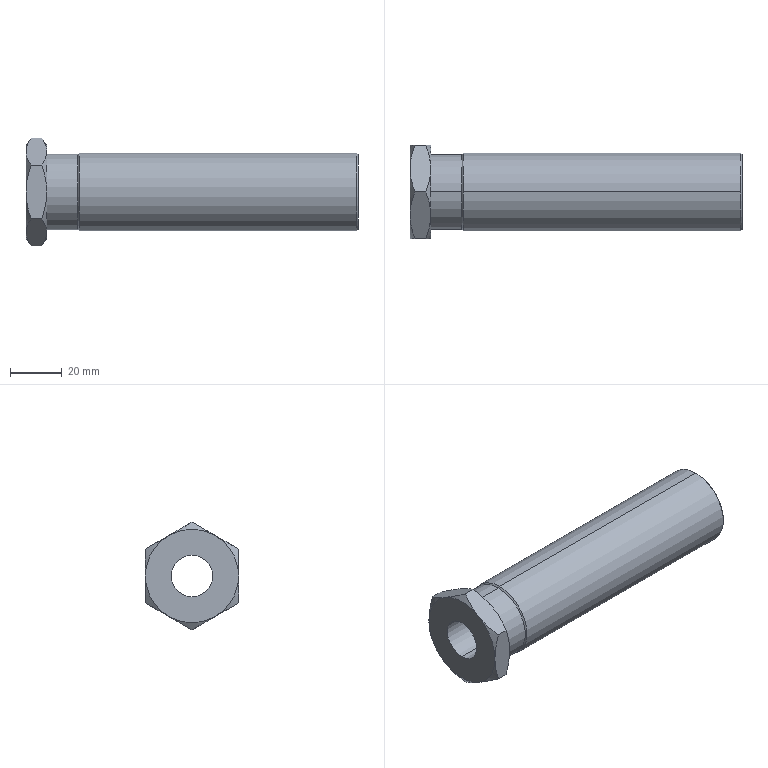Part | SolidWorks | features ICE 2, Extrusion 1, RevCut 1, Revolution 1 | 1 solid | 32 faces | box 128 x 36 x 41.569 mm | volume 67364 mm3 | cone 17 | plane 9 | cylinder 6 | commonest cylinder face diameters 16 x2 29 x2 30 x2
STEP:
#1=CARTESIAN_POINT('',(120.,0.,-8.));
#2=VERTEX_POINT('',#1);
#3=CARTESIAN_POINT('',(120.,0.,8.));
#4=VERTEX_POINT('',#3);
#5=CARTESIAN_POINT('',(120.,0.,0.));
#6=DIRECTION('',(-1.,0.,0.));
#7=DIRECTION('',(0.,0.,1.));
#8=AXIS2_PLACEMENT_3D('',#5,#6,#7);
#9=CIRCLE('',#8,8.);
#10=EDGE_CURVE('',#2,#4,#9,.T.);
#11=ORIENTED_EDGE('',*,*,#10,.F.);
#12=CARTESIAN_POINT('',(-8.,0.,-8.));
#13=VERTEX_POINT('',#12);
#14=CARTESIAN_POINT('',(0.,0.,-8.));
#15=DIRECTION('',(-1.,0.,0.));
#16=VECTOR('',#15,1000.);
#17=LINE('',#14,#16);
#18=EDGE_CURVE('',#2,#13,#17,.T.);
#19=ORIENTED_EDGE('',*,*,#18,.T.);
#20=CARTESIAN_POINT('',(-8.,0.,8.));
#21=VERTEX_POINT('',#20);
#22=CARTESIAN_POINT('',(-8.,0.,0.));
#23=DIRECTION('',(-1.,0.,0.));
#24=DIRECTION('',(0.,0.,1.));
#25=AXIS2_PLACEMENT_3D('',#22,#23,#24);
#26=CIRCLE('',#25,8.);
#27=EDGE_CURVE('',#13,#21,#26,.T.);
#28=ORIENTED_EDGE('',*,*,#27,.T.);
#29=CARTESIAN_POINT('',(0.,0.,8.));
#30=DIRECTION('',(-1.,0.,0.));
#31=VECTOR('',#30,1000.);
#32=LINE('',#29,#31);
#33=EDGE_CURVE('',#4,#21,#32,.T.);
#34=ORIENTED_EDGE('',*,*,#33,.F.);
#35=EDGE_LOOP('',(#11,#19,#28,#34));
#36=FACE_OUTER_BOUND('',#35,.T.);
#37=CARTESIAN_POINT('',(0.,0.,0.));
#38=DIRECTION('',(-1.,0.,0.));
#39=DIRECTION('',(0.,0.,1.));
#40=AXIS2_PLACEMENT_3D('',#37,#38,#39);
#41=CYLINDRICAL_SURFACE('',#40,8.);
#42=ADVANCED_FACE('',(#36),#41,.F.);
#43=CARTESIAN_POINT('',(0.,9.,-15.588));
#44=VERTEX_POINT('',#43);
#45=CARTESIAN_POINT('',(0.,0.,-18.));
#46=VERTEX_POINT('',#45);
#47=CARTESIAN_POINT('',(0.,0.,0.));
#48=DIRECTION('',(-1.,0.,0.));
#49=DIRECTION('',(0.,0.,1.));
#50=AXIS2_PLACEMENT_3D('',#47,#48,#49);
#51=CIRCLE('',#50,18.);
#52=EDGE_CURVE('',#44,#46,#51,.T.);
#53=ORIENTED_EDGE('',*,*,#52,.T.);
#54=CARTESIAN_POINT('',(-1.95,0.,-20.785));
#55=VERTEX_POINT('',#54);
#56=CARTESIAN_POINT('',(0.,0.,-18.));
#57=DIRECTION('',(-0.5736,0.,-0.8192));
#58=VECTOR('',#57,1000.);
#59=LINE('',#56,#58);
#60=EDGE_CURVE('',#46,#55,#59,.T.);
#61=ORIENTED_EDGE('',*,*,#60,.T.);
#62=CARTESIAN_POINT('',(-1.95,0.,-20.785));
#63=CARTESIAN_POINT('',(-1.359,1.461,-19.941));
#64=CARTESIAN_POINT('',(-0.8697,2.937,-19.089));
#65=CARTESIAN_POINT('',(-0.189,5.933,-17.359));
#66=CARTESIAN_POINT('',(0.,7.453,-16.482));
#67=CARTESIAN_POINT('',(0.,9.,-15.588));
#68=B_SPLINE_CURVE_WITH_KNOTS('',3,(#62,#63,#64,#65,#66,#67),.UNSPECIFIED.,.F.,.F.,(4,2,4),(0.000000241,0.005286,0.01057),.UNSPECIFIED.);
#69=EDGE_CURVE('',#55,#44,#68,.T.);
#70=ORIENTED_EDGE('',*,*,#69,.T.);
#71=EDGE_LOOP('',(#53,#61,#70));
#72=FACE_OUTER_BOUND('',#71,.T.);
#73=CARTESIAN_POINT('',(0.,0.,0.));
#74=DIRECTION('',(-1.,0.,0.));
#75=DIRECTION('',(0.,0.,-1.));
#76=AXIS2_PLACEMENT_3D('',#73,#74,#75);
#77=CONICAL_SURFACE('',#76,18.,0.9599);
#78=ADVANCED_FACE('',(#72),#77,.T.);
#79=CARTESIAN_POINT('',(12.,0.,14.5));
#80=VERTEX_POINT('',#79);
#81=CARTESIAN_POINT('',(12.,0.,-14.5));
#82=VERTEX_POINT('',#81);
#83=CARTESIAN_POINT('',(12.,0.,0.));
#84=DIRECTION('',(-1.,0.,0.));
#85=DIRECTION('',(0.,0.,1.));
#86=AXIS2_PLACEMENT_3D('',#83,#84,#85);
#87=CIRCLE('',#86,14.5);
#88=EDGE_CURVE('',#80,#82,#87,.T.);
#89=ORIENTED_EDGE('',*,*,#88,.T.);
#90=CARTESIAN_POINT('',(0.,0.,-14.5));
#91=VERTEX_POINT('',#90);
#92=CARTESIAN_POINT('',(0.,0.,-14.5));
#93=DIRECTION('',(-1.,0.,0.));
#94=VECTOR('',#93,1000.);
#95=LINE('',#92,#94);
#96=EDGE_CURVE('',#82,#91,#95,.T.);
#97=ORIENTED_EDGE('',*,*,#96,.T.);
#98=CARTESIAN_POINT('',(0.,0.,14.5));
#99=VERTEX_POINT('',#98);
#100=CARTESIAN_POINT('',(0.,0.,0.));
#101=DIRECTION('',(-1.,0.,0.));
#102=DIRECTION('',(0.,0.,1.));
#103=AXIS2_PLACEMENT_3D('',#100,#101,#102);
#104=CIRCLE('',#103,14.5);
#105=EDGE_CURVE('',#99,#91,#104,.T.);
#106=ORIENTED_EDGE('',*,*,#105,.F.);
#107=CARTESIAN_POINT('',(0.,0.,14.5));
#108=DIRECTION('',(-1.,0.,0.));
#109=VECTOR('',#108,1000.);
#110=LINE('',#107,#109);
#111=EDGE_CURVE('',#80,#99,#110,.T.);
#112=ORIENTED_EDGE('',*,*,#111,.F.);
#113=EDGE_LOOP('',(#89,#97,#106,#112));
#114=FACE_OUTER_BOUND('',#113,.T.);
#115=CARTESIAN_POINT('',(0.,0.,0.));
#116=DIRECTION('',(-1.,0.,0.));
#117=DIRECTION('',(0.,0.,1.));
#118=AXIS2_PLACEMENT_3D('',#115,#116,#117);
#119=CYLINDRICAL_SURFACE('',#118,14.5);
#120=ADVANCED_FACE('',(#114),#119,.T.);
#121=ORIENTED_EDGE('',*,*,#88,.F.);
#122=CARTESIAN_POINT('',(12.5,0.,15.));
#123=VERTEX_POINT('',#122);
#124=CARTESIAN_POINT('',(12.5,0.,15.));
#125=DIRECTION('',(0.7071,0.,0.7071));
#126=VECTOR('',#125,1000.);
#127=LINE('',#124,#126);
#128=EDGE_CURVE('',#80,#123,#127,.T.);
#129=ORIENTED_EDGE('',*,*,#128,.T.);
#130=CARTESIAN_POINT('',(12.5,0.,-15.));
#131=VERTEX_POINT('',#130);
#132=CARTESIAN_POINT('',(12.5,0.,0.));
#133=DIRECTION('',(-1.,0.,0.));
#134=DIRECTION('',(0.,0.,1.));
#135=AXIS2_PLACEMENT_3D('',#132,#133,#134);
#136=CIRCLE('',#135,15.);
#137=EDGE_CURVE('',#123,#131,#136,.T.);
#138=ORIENTED_EDGE('',*,*,#137,.T.);
#139=CARTESIAN_POINT('',(12.5,0.,-15.));
#140=DIRECTION('',(0.7071,0.,-0.7071));
#141=VECTOR('',#140,1000.);
#142=LINE('',#139,#141);
#143=EDGE_CURVE('',#82,#131,#142,.T.);
#144=ORIENTED_EDGE('',*,*,#143,.F.);
#145=EDGE_LOOP('',(#121,#129,#138,#144));
#146=FACE_OUTER_BOUND('',#145,.T.);
#147=CARTESIAN_POINT('',(12.5,0.,0.));
#148=DIRECTION('',(1.,0.,0.));
#149=DIRECTION('',(0.,0.,-1.));
#150=AXIS2_PLACEMENT_3D('',#147,#148,#149);
#151=CONICAL_SURFACE('',#150,15.,0.7854);
#152=ADVANCED_FACE('',(#146),#151,.T.);
#153=CARTESIAN_POINT('',(119.5,0.,15.));
#154=VERTEX_POINT('',#153);
#155=CARTESIAN_POINT('',(119.5,0.,-15.));
#156=VERTEX_POINT('',#155);
#157=CARTESIAN_POINT('',(119.5,0.,0.));
#158=DIRECTION('',(-1.,0.,0.));
#159=DIRECTION('',(0.,0.,1.));
#160=AXIS2_PLACEMENT_3D('',#157,#158,#159);
#161=CIRCLE('',#160,15.);
#162=EDGE_CURVE('',#154,#156,#161,.T.);
#163=ORIENTED_EDGE('',*,*,#162,.T.);
#164=CARTESIAN_POINT('',(0.,0.,-15.));
#165=DIRECTION('',(-1.,0.,0.));
#166=VECTOR('',#165,1000.);
#167=LINE('',#164,#166);
#168=EDGE_CURVE('',#156,#131,#167,.T.);
#169=ORIENTED_EDGE('',*,*,#168,.T.);
#170=ORIENTED_EDGE('',*,*,#137,.F.);
#171=CARTESIAN_POINT('',(0.,0.,15.));
#172=DIRECTION('',(-1.,0.,0.));
#173=VECTOR('',#172,1000.);
#174=LINE('',#171,#173);
#175=EDGE_CURVE('',#154,#123,#174,.T.);
#176=ORIENTED_EDGE('',*,*,#175,.F.);
#177=EDGE_LOOP('',(#163,#169,#170,#176));
#178=FACE_OUTER_BOUND('',#177,.T.);
#179=CARTESIAN_POINT('',(0.,0.,0.));
#180=DIRECTION('',(-1.,0.,0.));
#181=DIRECTION('',(0.,0.,1.));
#182=AXIS2_PLACEMENT_3D('',#179,#180,#181);
#183=CYLINDRICAL_SURFACE('',#182,15.);
#184=ADVANCED_FACE('',(#178),#183,.T.);
#185=CARTESIAN_POINT('',(120.,0.,14.5));
#186=VERTEX_POINT('',#185);
#187=CARTESIAN_POINT('',(120.,0.,-14.5));
#188=VERTEX_POINT('',#187);
#189=CARTESIAN_POINT('',(120.,0.,0.));
#190=DIRECTION('',(-1.,0.,0.));
#191=DIRECTION('',(0.,0.,1.));
#192=AXIS2_PLACEMENT_3D('',#189,#190,#191);
#193=CIRCLE('',#192,14.5);
#194=EDGE_CURVE('',#186,#188,#193,.T.);
#195=ORIENTED_EDGE('',*,*,#194,.T.);
#196=CARTESIAN_POINT('',(120.,0.,-14.5));
#197=DIRECTION('',(-0.7071,0.,-0.7071));
#198=VECTOR('',#197,1000.);
#199=LINE('',#196,#198);
#200=EDGE_CURVE('',#188,#156,#199,.T.);
#201=ORIENTED_EDGE('',*,*,#200,.T.);
#202=ORIENTED_EDGE('',*,*,#162,.F.);
#203=CARTESIAN_POINT('',(120.,0.,14.5));
#204=DIRECTION('',(-0.7071,0.,0.7071));
#205=VECTOR('',#204,1000.);
#206=LINE('',#203,#205);
#207=EDGE_CURVE('',#186,#154,#206,.T.);
#208=ORIENTED_EDGE('',*,*,#207,.F.);
#209=EDGE_LOOP('',(#195,#201,#202,#208));
#210=FACE_OUTER_BOUND('',#209,.T.);
#211=CARTESIAN_POINT('',(120.,0.,0.));
#212=DIRECTION('',(-1.,0.,0.));
#213=DIRECTION('',(0.,0.,1.));
#214=AXIS2_PLACEMENT_3D('',#211,#212,#213);
#215=CONICAL_SURFACE('',#214,14.5,0.7854);
#216=ADVANCED_FACE('',(#210),#215,.T.);
#217=ORIENTED_EDGE('',*,*,#194,.F.);
#218=CARTESIAN_POINT('',(120.,0.,0.));
#219=DIRECTION('',(-1.,0.,0.));
#220=DIRECTION('',(0.,0.,1.));
#221=AXIS2_PLACEMENT_3D('',#218,#219,#220);
#222=CIRCLE('',#221,14.5);
#223=EDGE_CURVE('',#188,#186,#222,.T.);
#224=ORIENTED_EDGE('',*,*,#223,.F.);
#225=EDGE_LOOP('',(#217,#224));
#226=FACE_OUTER_BOUND('',#225,.T.);
#227=CARTESIAN_POINT('',(120.,0.,0.));
#228=DIRECTION('',(-1.,0.,0.));
#229=DIRECTION('',(0.,0.,1.));
#230=AXIS2_PLACEMENT_3D('',#227,#228,#229);
#231=CIRCLE('',#230,8.);
#232=EDGE_CURVE('',#4,#2,#231,.T.);
#233=ORIENTED_EDGE('',*,*,#232,.T.);
#234=ORIENTED_EDGE('',*,*,#10,.T.);
#235=EDGE_LOOP('',(#233,#234));
#236=FACE_BOUND('',#235,.T.);
#237=CARTESIAN_POINT('',(120.,0.,0.));
#238=DIRECTION('',(-1.,0.,0.));
#239=DIRECTION('',(0.,0.,1.));
#240=AXIS2_PLACEMENT_3D('',#237,#238,#239);
#241=PLANE('',#240);
#242=ADVANCED_FACE('',(#226,#236),#241,.F.);
#243=CARTESIAN_POINT('',(-8.,-9.,15.588));
#244=VERTEX_POINT('',#243);
#245=CARTESIAN_POINT('',(-8.,9.,15.588));
#246=VERTEX_POINT('',#245);
#247=CARTESIAN_POINT('',(-8.,0.,0.));
#248=DIRECTION('',(-1.,0.,0.));
#249=DIRECTION('',(0.,0.,1.));
#250=AXIS2_PLACEMENT_3D('',#247,#248,#249);
#251=CIRCLE('',#250,18.);
#252=EDGE_CURVE('',#244,#246,#251,.T.);
#253=ORIENTED_EDGE('',*,*,#252,.T.);
#254=CARTESIAN_POINT('',(-8.,18.,0.));
#255=VERTEX_POINT('',#254);
#256=CARTESIAN_POINT('',(-8.,0.,0.));
#257=DIRECTION('',(-1.,0.,0.));
#258=DIRECTION('',(0.,0.,1.));
#259=AXIS2_PLACEMENT_3D('',#256,#257,#258);
#260=CIRCLE('',#259,18.);
#261=EDGE_CURVE('',#246,#255,#260,.T.);
#262=ORIENTED_EDGE('',*,*,#261,.T.);
#263=CARTESIAN_POINT('',(-8.,9.,-15.588));
#264=VERTEX_POINT('',#263);
#265=CARTESIAN_POINT('',(-8.,0.,0.));
#266=DIRECTION('',(-1.,0.,0.));
#267=DIRECTION('',(0.,0.,1.));
#268=AXIS2_PLACEMENT_3D('',#265,#266,#267);
#269=CIRCLE('',#268,18.);
#270=EDGE_CURVE('',#255,#264,#269,.T.);
#271=ORIENTED_EDGE('',*,*,#270,.T.);
#272=CARTESIAN_POINT('',(-8.,-9.,-15.588));
#273=VERTEX_POINT('',#272);
#274=CARTESIAN_POINT('',(-8.,0.,0.));
#275=DIRECTION('',(-1.,0.,0.));
#276=DIRECTION('',(0.,0.,1.));
#277=AXIS2_PLACEMENT_3D('',#274,#275,#276);
#278=CIRCLE('',#277,18.);
#279=EDGE_CURVE('',#264,#273,#278,.T.);
#280=ORIENTED_EDGE('',*,*,#279,.T.);
#281=CARTESIAN_POINT('',(-8.,-18.,0.));
#282=VERTEX_POINT('',#281);
#283=CARTESIAN_POINT('',(-8.,0.,0.));
#284=DIRECTION('',(-1.,0.,0.));
#285=DIRECTION('',(0.,0.,1.));
#286=AXIS2_PLACEMENT_3D('',#283,#284,#285);
#287=CIRCLE('',#286,18.);
#288=EDGE_CURVE('',#273,#282,#287,.T.);
#289=ORIENTED_EDGE('',*,*,#288,.T.);
#290=CARTESIAN_POINT('',(-8.,0.,0.));
#291=DIRECTION('',(-1.,0.,0.));
#292=DIRECTION('',(0.,-1.,0.));
#293=AXIS2_PLACEMENT_3D('',#290,#291,#292);
#294=CIRCLE('',#293,18.);
#295=EDGE_CURVE('',#282,#244,#294,.T.);
#296=ORIENTED_EDGE('',*,*,#295,.T.);
#297=EDGE_LOOP('',(#253,#262,#271,#280,#289,#296));
#298=FACE_OUTER_BOUND('',#297,.T.);
#299=CARTESIAN_POINT('',(-8.,0.,0.));
#300=DIRECTION('',(-1.,0.,0.));
#301=DIRECTION('',(0.,0.,1.));
#302=AXIS2_PLACEMENT_3D('',#299,#300,#301);
#303=CIRCLE('',#302,8.);
#304=EDGE_CURVE('',#21,#13,#303,.T.);
#305=ORIENTED_EDGE('',*,*,#304,.F.);
#306=ORIENTED_EDGE('',*,*,#27,.F.);
#307=EDGE_LOOP('',(#305,#306));
#308=FACE_BOUND('',#307,.T.);
#309=CARTESIAN_POINT('',(-8.,0.,-20.785));
#310=DIRECTION('',(-1.,0.,0.));
#311=DIRECTION('',(0.,0.,1.));
#312=AXIS2_PLACEMENT_3D('',#309,#310,#311);
#313=PLANE('',#312);
#314=ADVANCED_FACE('',(#298,#308),#313,.T.);
#315=ORIENTED_EDGE('',*,*,#105,.T.);
#316=CARTESIAN_POINT('',(0.,0.,0.));
#317=DIRECTION('',(-1.,0.,0.));
#318=DIRECTION('',(0.,0.,1.));
#319=AXIS2_PLACEMENT_3D('',#316,#317,#318);
#320=CIRCLE('',#319,14.5);
#321=EDGE_CURVE('',#91,#99,#320,.T.);
#322=ORIENTED_EDGE('',*,*,#321,.T.);
#323=EDGE_LOOP('',(#315,#322));
#324=FACE_BOUND('',#323,.T.);
#325=CARTESIAN_POINT('',(0.,9.,15.588));
#326=VERTEX_POINT('',#325);
#327=CARTESIAN_POINT('',(0.,18.,0.));
#328=VERTEX_POINT('',#327);
#329=CARTESIAN_POINT('',(0.,0.,0.));
#330=DIRECTION('',(-1.,0.,0.));
#331=DIRECTION('',(0.,0.,1.));
#332=AXIS2_PLACEMENT_3D('',#329,#330,#331);
#333=CIRCLE('',#332,18.);
#334=EDGE_CURVE('',#326,#328,#333,.T.);
#335=ORIENTED_EDGE('',*,*,#334,.F.);
#336=CARTESIAN_POINT('',(0.,-9.,15.588));
#337=VERTEX_POINT('',#336);
#338=CARTESIAN_POINT('',(0.,0.,0.));
#339=DIRECTION('',(-1.,0.,0.));
#340=DIRECTION('',(0.,0.,1.));
#341=AXIS2_PLACEMENT_3D('',#338,#339,#340);
#342=CIRCLE('',#341,18.);
#343=EDGE_CURVE('',#337,#326,#342,.T.);
#344=ORIENTED_EDGE('',*,*,#343,.F.);
#345=CARTESIAN_POINT('',(0.,-18.,0.));
#346=VERTEX_POINT('',#345);
#347=CARTESIAN_POINT('',(0.,0.,0.));
#348=DIRECTION('',(-1.,0.,0.));
#349=DIRECTION('',(0.,0.,1.));
#350=AXIS2_PLACEMENT_3D('',#347,#348,#349);
#351=CIRCLE('',#350,18.);
#352=EDGE_CURVE('',#346,#337,#351,.T.);
#353=ORIENTED_EDGE('',*,*,#352,.F.);
#354=CARTESIAN_POINT('',(0.,-9.,-15.588));
#355=VERTEX_POINT('',#354);
#356=CARTESIAN_POINT('',(0.,0.,0.));
#357=DIRECTION('',(-1.,0.,0.));
#358=DIRECTION('',(0.,0.,1.));
#359=AXIS2_PLACEMENT_3D('',#356,#357,#358);
#360=CIRCLE('',#359,18.);
#361=EDGE_CURVE('',#355,#346,#360,.T.);
#362=ORIENTED_EDGE('',*,*,#361,.F.);
#363=CARTESIAN_POINT('',(0.,0.,0.));
#364=DIRECTION('',(-1.,0.,0.));
#365=DIRECTION('',(0.,0.,1.));
#366=AXIS2_PLACEMENT_3D('',#363,#364,#365);
#367=CIRCLE('',#366,18.);
#368=EDGE_CURVE('',#46,#355,#367,.T.);
#369=ORIENTED_EDGE('',*,*,#368,.F.);
#370=ORIENTED_EDGE('',*,*,#52,.F.);
#371=CARTESIAN_POINT('',(0.,0.,0.));
#372=DIRECTION('',(1.,0.,0.));
#373=DIRECTION('',(0.,0.,-1.));
#374=AXIS2_PLACEMENT_3D('',#371,#372,#373);
#375=CIRCLE('',#374,18.);
#376=EDGE_CURVE('',#44,#328,#375,.T.);
#377=ORIENTED_EDGE('',*,*,#376,.T.);
#378=EDGE_LOOP('',(#335,#344,#353,#362,#369,#370,#377));
#379=FACE_OUTER_BOUND('',#378,.T.);
#380=CARTESIAN_POINT('',(0.,0.,-20.785));
#381=DIRECTION('',(-1.,0.,0.));
#382=DIRECTION('',(0.,0.,1.));
#383=AXIS2_PLACEMENT_3D('',#380,#381,#382);
#384=PLANE('',#383);
#385=ADVANCED_FACE('',(#324,#379),#384,.F.);
#386=ORIENTED_EDGE('',*,*,#200,.F.);
#387=ORIENTED_EDGE('',*,*,#223,.T.);
#388=ORIENTED_EDGE('',*,*,#207,.T.);
#389=CARTESIAN_POINT('',(119.5,0.,0.));
#390=DIRECTION('',(-1.,0.,0.));
#391=DIRECTION('',(0.,0.,1.));
#392=AXIS2_PLACEMENT_3D('',#389,#390,#391);
#393=CIRCLE('',#392,15.);
#394=EDGE_CURVE('',#156,#154,#393,.T.);
#395=ORIENTED_EDGE('',*,*,#394,.F.);
#396=EDGE_LOOP('',(#386,#387,#388,#395));
#397=FACE_OUTER_BOUND('',#396,.T.);
#398=CARTESIAN_POINT('',(120.,0.,0.));
#399=DIRECTION('',(-1.,0.,0.));
#400=DIRECTION('',(0.,0.,1.));
#401=AXIS2_PLACEMENT_3D('',#398,#399,#400);
#402=CONICAL_SURFACE('',#401,14.5,0.7854);
#403=ADVANCED_FACE('',(#397),#402,.T.);
#404=ORIENTED_EDGE('',*,*,#168,.F.);
#405=ORIENTED_EDGE('',*,*,#394,.T.);
#406=ORIENTED_EDGE('',*,*,#175,.T.);
#407=CARTESIAN_POINT('',(12.5,0.,0.));
#408=DIRECTION('',(-1.,0.,0.));
#409=DIRECTION('',(0.,0.,1.));
#410=AXIS2_PLACEMENT_3D('',#407,#408,#409);
#411=CIRCLE('',#410,15.);
#412=EDGE_CURVE('',#131,#123,#411,.T.);
#413=ORIENTED_EDGE('',*,*,#412,.F.);
#414=EDGE_LOOP('',(#404,#405,#406,#413));
#415=FACE_OUTER_BOUND('',#414,.T.);
#416=CARTESIAN_POINT('',(0.,0.,0.));
#417=DIRECTION('',(-1.,0.,0.));
#418=DIRECTION('',(0.,0.,1.));
#419=AXIS2_PLACEMENT_3D('',#416,#417,#418);
#420=CYLINDRICAL_SURFACE('',#419,15.);
#421=ADVANCED_FACE('',(#415),#420,.T.);
#422=ORIENTED_EDGE('',*,*,#128,.F.);
#423=CARTESIAN_POINT('',(12.,0.,0.));
#424=DIRECTION('',(-1.,0.,0.));
#425=DIRECTION('',(0.,0.,1.));
#426=AXIS2_PLACEMENT_3D('',#423,#424,#425);
#427=CIRCLE('',#426,14.5);
#428=EDGE_CURVE('',#82,#80,#427,.T.);
#429=ORIENTED_EDGE('',*,*,#428,.F.);
#430=ORIENTED_EDGE('',*,*,#143,.T.);
#431=ORIENTED_EDGE('',*,*,#412,.T.);
#432=EDGE_LOOP('',(#422,#429,#430,#431));
#433=FACE_OUTER_BOUND('',#432,.T.);
#434=CARTESIAN_POINT('',(12.5,0.,0.));
#435=DIRECTION('',(1.,0.,0.));
#436=DIRECTION('',(0.,0.,-1.));
#437=AXIS2_PLACEMENT_3D('',#434,#435,#436);
#438=CONICAL_SURFACE('',#437,15.,0.7854);
#439=ADVANCED_FACE('',(#433),#438,.T.);
#440=ORIENTED_EDGE('',*,*,#96,.F.);
#441=ORIENTED_EDGE('',*,*,#428,.T.);
#442=ORIENTED_EDGE('',*,*,#111,.T.);
#443=ORIENTED_EDGE('',*,*,#321,.F.);
#444=EDGE_LOOP('',(#440,#441,#442,#443));
#445=FACE_OUTER_BOUND('',#444,.T.);
#446=CARTESIAN_POINT('',(0.,0.,0.));
#447=DIRECTION('',(-1.,0.,0.));
#448=DIRECTION('',(0.,0.,1.));
#449=AXIS2_PLACEMENT_3D('',#446,#447,#448);
#450=CYLINDRICAL_SURFACE('',#449,14.5);
#451=ADVANCED_FACE('',(#445),#450,.T.);
#452=CARTESIAN_POINT('',(-1.95,0.,20.785));
#453=VERTEX_POINT('',#452);
#454=CARTESIAN_POINT('',(-1.95,0.,20.785));
#455=CARTESIAN_POINT('',(-1.359,-1.461,19.941));
#456=CARTESIAN_POINT('',(-0.8697,-2.937,19.089));
#457=CARTESIAN_POINT('',(-0.189,-5.933,17.359));
#458=CARTESIAN_POINT('',(0.,-7.453,16.482));
#459=CARTESIAN_POINT('',(0.,-9.,15.588));
#460=B_SPLINE_CURVE_WITH_KNOTS('',3,(#454,#455,#456,#457,#458,#459),.UNSPECIFIED.,.F.,.F.,(4,2,4),(0.000000241,0.005286,0.01057),.UNSPECIFIED.);
#461=EDGE_CURVE('',#453,#337,#460,.T.);
#462=ORIENTED_EDGE('',*,*,#461,.T.);
#463=ORIENTED_EDGE('',*,*,#343,.T.);
#464=CARTESIAN_POINT('',(0.,9.,15.588));
#465=CARTESIAN_POINT('',(0.,8.616,15.81));
#466=CARTESIAN_POINT('',(-0.01156,8.229,16.033));
#467=CARTESIAN_POINT('',(-0.0577,7.458,16.479));
#468=CARTESIAN_POINT('',(-0.09213,7.074,16.7));
#469=CARTESIAN_POINT('',(-0.2277,5.929,17.361));
#470=CARTESIAN_POINT('',(-0.3612,5.173,17.798));
#471=CARTESIAN_POINT('',(-0.8729,2.926,19.095));
#472=CARTESIAN_POINT('',(-1.362,1.454,19.945));
#473=CARTESIAN_POINT('',(-1.95,0.,20.785));
#474=B_SPLINE_CURVE_WITH_KNOTS('',3,(#464,#465,#466,#467,#468,#469,#470,#471,#472,#473),.UNSPECIFIED.,.F.,.F.,(4,2,2,2,4),(0.01057,0.01188,0.0132,0.01582,0.02106),.UNSPECIFIED.);
#475=EDGE_CURVE('',#326,#453,#474,.T.);
#476=ORIENTED_EDGE('',*,*,#475,.T.);
#477=EDGE_LOOP('',(#462,#463,#476));
#478=FACE_OUTER_BOUND('',#477,.T.);
#479=CARTESIAN_POINT('',(0.,0.,0.));
#480=DIRECTION('',(-1.,0.,0.));
#481=DIRECTION('',(0.,0.,-1.));
#482=AXIS2_PLACEMENT_3D('',#479,#480,#481);
#483=CONICAL_SURFACE('',#482,18.,0.9599);
#484=ADVANCED_FACE('',(#478),#483,.T.);
#485=CARTESIAN_POINT('',(-1.95,-18.,10.392));
#486=VERTEX_POINT('',#485);
#487=CARTESIAN_POINT('',(-1.95,-18.,10.392));
#488=CARTESIAN_POINT('',(-1.366,-18.,8.725));
#489=CARTESIAN_POINT('',(-0.8773,-18.,7.032));
#490=CARTESIAN_POINT('',(-0.363,-18.,4.43));
#491=CARTESIAN_POINT('',(-0.2283,-18.,3.552));
#492=CARTESIAN_POINT('',(-0.04592,-18.,1.772));
#493=CARTESIAN_POINT('',(0.,-18.,0.883));
#494=CARTESIAN_POINT('',(0.,-18.,0.));
#495=B_SPLINE_CURVE_WITH_KNOTS('',3,(#487,#488,#489,#490,#491,#492,#493,#494),.UNSPECIFIED.,.F.,.F.,(4,2,2,4),(0.04198,0.04728,0.04992,0.05257),.UNSPECIFIED.);
#496=EDGE_CURVE('',#486,#346,#495,.T.);
#497=ORIENTED_EDGE('',*,*,#496,.T.);
#498=ORIENTED_EDGE('',*,*,#352,.T.);
#499=CARTESIAN_POINT('',(0.,-9.,15.588));
#500=CARTESIAN_POINT('',(0.,-9.384,15.367));
#501=CARTESIAN_POINT('',(-0.01156,-9.771,15.143));
#502=CARTESIAN_POINT('',(-0.0577,-10.542,14.698));
#503=CARTESIAN_POINT('',(-0.09213,-10.926,14.477));
#504=CARTESIAN_POINT('',(-0.2277,-12.071,13.816));
#505=CARTESIAN_POINT('',(-0.3612,-12.827,13.379));
#506=CARTESIAN_POINT('',(-0.8729,-15.074,12.082));
#507=CARTESIAN_POINT('',(-1.362,-16.546,11.232));
#508=CARTESIAN_POINT('',(-1.95,-18.,10.392));
#509=B_SPLINE_CURVE_WITH_KNOTS('',3,(#499,#500,#501,#502,#503,#504,#505,#506,#507,#508),.UNSPECIFIED.,.F.,.F.,(4,2,2,2,4),(0.01057,0.01188,0.0132,0.01582,0.02106),.UNSPECIFIED.);
#510=EDGE_CURVE('',#337,#486,#509,.T.);
#511=ORIENTED_EDGE('',*,*,#510,.T.);
#512=EDGE_LOOP('',(#497,#498,#511));
#513=FACE_OUTER_BOUND('',#512,.T.);
#514=CARTESIAN_POINT('',(0.,0.,0.));
#515=DIRECTION('',(-1.,0.,0.));
#516=DIRECTION('',(0.,0.,-1.));
#517=AXIS2_PLACEMENT_3D('',#514,#515,#516);
#518=CONICAL_SURFACE('',#517,18.,0.9599);
#519=ADVANCED_FACE('',(#513),#518,.T.);
#520=CARTESIAN_POINT('',(-1.95,-18.,-10.392));
#521=VERTEX_POINT('',#520);
#522=CARTESIAN_POINT('',(0.,-18.,0.));
#523=CARTESIAN_POINT('',(0.,-18.,-1.769));
#524=CARTESIAN_POINT('',(-0.1856,-18.,-3.52));
#525=CARTESIAN_POINT('',(-0.6966,-18.,-6.124));
#526=CARTESIAN_POINT('',(-0.9053,-18.,-6.988));
#527=CARTESIAN_POINT('',(-1.387,-18.,-8.709));
#528=CARTESIAN_POINT('',(-1.657,-18.,-9.556));
#529=CARTESIAN_POINT('',(-1.95,-18.,-10.392));
#530=B_SPLINE_CURVE_WITH_KNOTS('',3,(#522,#523,#524,#525,#526,#527,#528,#529),.UNSPECIFIED.,.F.,.F.,(4,2,2,4),(0.05257,0.05787,0.06052,0.06317),.UNSPECIFIED.);
#531=EDGE_CURVE('',#346,#521,#530,.T.);
#532=ORIENTED_EDGE('',*,*,#531,.T.);
#533=CARTESIAN_POINT('',(-1.95,-18.,-10.392));
#534=CARTESIAN_POINT('',(-1.359,-16.539,-11.236));
#535=CARTESIAN_POINT('',(-0.8697,-15.063,-12.088));
#536=CARTESIAN_POINT('',(-0.189,-12.067,-13.818));
#537=CARTESIAN_POINT('',(0.,-10.547,-14.695));
#538=CARTESIAN_POINT('',(0.,-9.,-15.588));
#539=B_SPLINE_CURVE_WITH_KNOTS('',3,(#533,#534,#535,#536,#537,#538),.UNSPECIFIED.,.F.,.F.,(4,2,4),(0.000000241,0.005286,0.01057),.UNSPECIFIED.);
#540=EDGE_CURVE('',#521,#355,#539,.T.);
#541=ORIENTED_EDGE('',*,*,#540,.T.);
#542=ORIENTED_EDGE('',*,*,#361,.T.);
#543=EDGE_LOOP('',(#532,#541,#542));
#544=FACE_OUTER_BOUND('',#543,.T.);
#545=CARTESIAN_POINT('',(0.,0.,0.));
#546=DIRECTION('',(-1.,0.,0.));
#547=DIRECTION('',(0.,0.,-1.));
#548=AXIS2_PLACEMENT_3D('',#545,#546,#547);
#549=CONICAL_SURFACE('',#548,18.,0.9599);
#550=ADVANCED_FACE('',(#544),#549,.T.);
#551=ORIENTED_EDGE('',*,*,#60,.F.);
#552=ORIENTED_EDGE('',*,*,#368,.T.);
#553=CARTESIAN_POINT('',(0.,-9.,-15.588));
#554=CARTESIAN_POINT('',(0.,-8.616,-15.81));
#555=CARTESIAN_POINT('',(-0.01156,-8.229,-16.033));
#556=CARTESIAN_POINT('',(-0.0577,-7.458,-16.479));
#557=CARTESIAN_POINT('',(-0.09213,-7.074,-16.7));
#558=CARTESIAN_POINT('',(-0.2277,-5.929,-17.361));
#559=CARTESIAN_POINT('',(-0.3612,-5.173,-17.798));
#560=CARTESIAN_POINT('',(-0.8729,-2.926,-19.095));
#561=CARTESIAN_POINT('',(-1.362,-1.454,-19.945));
#562=CARTESIAN_POINT('',(-1.95,0.,-20.785));
#563=B_SPLINE_CURVE_WITH_KNOTS('',3,(#553,#554,#555,#556,#557,#558,#559,#560,#561,#562),.UNSPECIFIED.,.F.,.F.,(4,2,2,2,4),(0.01057,0.01188,0.0132,0.01582,0.02106),.UNSPECIFIED.);
#564=EDGE_CURVE('',#355,#55,#563,.T.);
#565=ORIENTED_EDGE('',*,*,#564,.T.);
#566=EDGE_LOOP('',(#551,#552,#565));
#567=FACE_OUTER_BOUND('',#566,.T.);
#568=CARTESIAN_POINT('',(0.,0.,0.));
#569=DIRECTION('',(-1.,0.,0.));
#570=DIRECTION('',(0.,0.,-1.));
#571=AXIS2_PLACEMENT_3D('',#568,#569,#570);
#572=CONICAL_SURFACE('',#571,18.,0.9599);
#573=ADVANCED_FACE('',(#567),#572,.T.);
#574=CARTESIAN_POINT('',(-1.95,18.,-10.392));
#575=VERTEX_POINT('',#574);
#576=CARTESIAN_POINT('',(0.,9.,-15.588));
#577=CARTESIAN_POINT('',(0.,9.384,-15.367));
#578=CARTESIAN_POINT('',(-0.01156,9.771,-15.143));
#579=CARTESIAN_POINT('',(-0.0577,10.542,-14.698));
#580=CARTESIAN_POINT('',(-0.09213,10.926,-14.477));
#581=CARTESIAN_POINT('',(-0.2277,12.071,-13.816));
#582=CARTESIAN_POINT('',(-0.3612,12.827,-13.379));
#583=CARTESIAN_POINT('',(-0.8729,15.074,-12.082));
#584=CARTESIAN_POINT('',(-1.362,16.546,-11.232));
#585=CARTESIAN_POINT('',(-1.95,18.,-10.392));
#586=B_SPLINE_CURVE_WITH_KNOTS('',3,(#576,#577,#578,#579,#580,#581,#582,#583,#584,#585),.UNSPECIFIED.,.F.,.F.,(4,2,2,2,4),(0.01057,0.01188,0.0132,0.01582,0.02106),.UNSPECIFIED.);
#587=EDGE_CURVE('',#44,#575,#586,.T.);
#588=ORIENTED_EDGE('',*,*,#587,.T.);
#589=CARTESIAN_POINT('',(-1.95,18.,-10.392));
#590=CARTESIAN_POINT('',(-1.657,18.,-9.556));
#591=CARTESIAN_POINT('',(-1.387,18.,-8.709));
#592=CARTESIAN_POINT('',(-0.9053,18.,-6.988));
#593=CARTESIAN_POINT('',(-0.6966,18.,-6.124));
#594=CARTESIAN_POINT('',(-0.1856,18.,-3.52));
#595=CARTESIAN_POINT('',(0.,18.,-1.769));
#596=CARTESIAN_POINT('',(0.,18.,0.));
#597=B_SPLINE_CURVE_WITH_KNOTS('',3,(#589,#590,#591,#592,#593,#594,#595,#596),.UNSPECIFIED.,.F.,.F.,(4,2,2,4),(0.01663,0.01928,0.02192,0.02722),.UNSPECIFIED.);
#598=EDGE_CURVE('',#575,#328,#597,.T.);
#599=ORIENTED_EDGE('',*,*,#598,.T.);
#600=ORIENTED_EDGE('',*,*,#376,.F.);
#601=EDGE_LOOP('',(#588,#599,#600));
#602=FACE_OUTER_BOUND('',#601,.T.);
#603=CARTESIAN_POINT('',(0.,0.,0.));
#604=DIRECTION('',(-1.,0.,0.));
#605=DIRECTION('',(0.,0.,-1.));
#606=AXIS2_PLACEMENT_3D('',#603,#604,#605);
#607=CONICAL_SURFACE('',#606,18.,0.9599);
#608=ADVANCED_FACE('',(#602),#607,.T.);
#609=CARTESIAN_POINT('',(-1.95,18.,10.392));
#610=VERTEX_POINT('',#609);
#611=CARTESIAN_POINT('',(-1.95,18.,10.392));
#612=CARTESIAN_POINT('',(-1.359,16.539,11.236));
#613=CARTESIAN_POINT('',(-0.8697,15.063,12.088));
#614=CARTESIAN_POINT('',(-0.189,12.067,13.818));
#615=CARTESIAN_POINT('',(0.,10.547,14.695));
#616=CARTESIAN_POINT('',(0.,9.,15.588));
#617=B_SPLINE_CURVE_WITH_KNOTS('',3,(#611,#612,#613,#614,#615,#616),.UNSPECIFIED.,.F.,.F.,(4,2,4),(0.000000241,0.005286,0.01057),.UNSPECIFIED.);
#618=EDGE_CURVE('',#610,#326,#617,.T.);
#619=ORIENTED_EDGE('',*,*,#618,.T.);
#620=ORIENTED_EDGE('',*,*,#334,.T.);
#621=CARTESIAN_POINT('',(0.,18.,0.));
#622=CARTESIAN_POINT('',(0.,18.,0.883));
#623=CARTESIAN_POINT('',(-0.04592,18.,1.772));
#624=CARTESIAN_POINT('',(-0.2283,18.,3.552));
#625=CARTESIAN_POINT('',(-0.363,18.,4.43));
#626=CARTESIAN_POINT('',(-0.8773,18.,7.032));
#627=CARTESIAN_POINT('',(-1.366,18.,8.725));
#628=CARTESIAN_POINT('',(-1.95,18.,10.392));
#629=B_SPLINE_CURVE_WITH_KNOTS('',3,(#621,#622,#623,#624,#625,#626,#627,#628),.UNSPECIFIED.,.F.,.F.,(4,2,2,4),(0.02722,0.02986,0.03251,0.03779),.UNSPECIFIED.);
#630=EDGE_CURVE('',#328,#610,#629,.T.);
#631=ORIENTED_EDGE('',*,*,#630,.T.);
#632=EDGE_LOOP('',(#619,#620,#631));
#633=FACE_OUTER_BOUND('',#632,.T.);
#634=CARTESIAN_POINT('',(0.,0.,0.));
#635=DIRECTION('',(-1.,0.,0.));
#636=DIRECTION('',(0.,0.,-1.));
#637=AXIS2_PLACEMENT_3D('',#634,#635,#636);
#638=CONICAL_SURFACE('',#637,18.,0.9599);
#639=ADVANCED_FACE('',(#633),#638,.T.);
#640=CARTESIAN_POINT('',(-6.05,0.,-20.785));
#641=VERTEX_POINT('',#640);
#642=CARTESIAN_POINT('',(-8.,9.,-15.588));
#643=CARTESIAN_POINT('',(-8.,8.616,-15.81));
#644=CARTESIAN_POINT('',(-7.988,8.229,-16.033));
#645=CARTESIAN_POINT('',(-7.942,7.458,-16.479));
#646=CARTESIAN_POINT('',(-7.908,7.074,-16.7));
#647=CARTESIAN_POINT('',(-7.772,5.929,-17.361));
#648=CARTESIAN_POINT('',(-7.639,5.173,-17.798));
#649=CARTESIAN_POINT('',(-7.127,2.926,-19.095));
#650=CARTESIAN_POINT('',(-6.638,1.454,-19.945));
#651=CARTESIAN_POINT('',(-6.05,0.,-20.785));
#652=B_SPLINE_CURVE_WITH_KNOTS('',3,(#642,#643,#644,#645,#646,#647,#648,#649,#650,#651),.UNSPECIFIED.,.F.,.F.,(4,2,2,2,4),(0.01057,0.01188,0.0132,0.01582,0.02106),.UNSPECIFIED.);
#653=EDGE_CURVE('',#264,#641,#652,.T.);
#654=ORIENTED_EDGE('',*,*,#653,.T.);
#655=CARTESIAN_POINT('',(-6.05,0.,-20.785));
#656=CARTESIAN_POINT('',(-6.641,-1.461,-19.941));
#657=CARTESIAN_POINT('',(-7.13,-2.937,-19.089));
#658=CARTESIAN_POINT('',(-7.811,-5.933,-17.359));
#659=CARTESIAN_POINT('',(-8.,-7.453,-16.482));
#660=CARTESIAN_POINT('',(-8.,-9.,-15.588));
#661=B_SPLINE_CURVE_WITH_KNOTS('',3,(#655,#656,#657,#658,#659,#660),.UNSPECIFIED.,.F.,.F.,(4,2,4),(0.000000241,0.005286,0.01057),.UNSPECIFIED.);
#662=EDGE_CURVE('',#641,#273,#661,.T.);
#663=ORIENTED_EDGE('',*,*,#662,.T.);
#664=ORIENTED_EDGE('',*,*,#279,.F.);
#665=EDGE_LOOP('',(#654,#663,#664));
#666=FACE_OUTER_BOUND('',#665,.T.);
#667=CARTESIAN_POINT('',(-8.,0.,0.));
#668=DIRECTION('',(1.,0.,0.));
#669=DIRECTION('',(0.,-1.,0.));
#670=AXIS2_PLACEMENT_3D('',#667,#668,#669);
#671=CONICAL_SURFACE('',#670,18.,0.9599);
#672=ADVANCED_FACE('',(#666),#671,.T.);
#673=CARTESIAN_POINT('',(-6.05,-18.,-10.392));
#674=VERTEX_POINT('',#673);
#675=CARTESIAN_POINT('',(-8.,-9.,-15.588));
#676=CARTESIAN_POINT('',(-8.,-9.384,-15.367));
#677=CARTESIAN_POINT('',(-7.988,-9.771,-15.143));
#678=CARTESIAN_POINT('',(-7.942,-10.542,-14.698));
#679=CARTESIAN_POINT('',(-7.908,-10.926,-14.477));
#680=CARTESIAN_POINT('',(-7.772,-12.071,-13.816));
#681=CARTESIAN_POINT('',(-7.639,-12.827,-13.379));
#682=CARTESIAN_POINT('',(-7.127,-15.074,-12.082));
#683=CARTESIAN_POINT('',(-6.638,-16.546,-11.232));
#684=CARTESIAN_POINT('',(-6.05,-18.,-10.392));
#685=B_SPLINE_CURVE_WITH_KNOTS('',3,(#675,#676,#677,#678,#679,#680,#681,#682,#683,#684),.UNSPECIFIED.,.F.,.F.,(4,2,2,2,4),(0.01057,0.01188,0.0132,0.01582,0.02106),.UNSPECIFIED.);
#686=EDGE_CURVE('',#273,#674,#685,.T.);
#687=ORIENTED_EDGE('',*,*,#686,.T.);
#688=CARTESIAN_POINT('',(-6.05,-18.,-10.392));
#689=CARTESIAN_POINT('',(-6.343,-18.,-9.556));
#690=CARTESIAN_POINT('',(-6.613,-18.,-8.709));
#691=CARTESIAN_POINT('',(-7.095,-18.,-6.988));
#692=CARTESIAN_POINT('',(-7.303,-18.,-6.123));
#693=CARTESIAN_POINT('',(-7.814,-18.,-3.52));
#694=CARTESIAN_POINT('',(-8.,-18.,-1.769));
#695=CARTESIAN_POINT('',(-8.,-18.,0.));
#696=B_SPLINE_CURVE_WITH_KNOTS('',3,(#688,#689,#690,#691,#692,#693,#694,#695),.UNSPECIFIED.,.F.,.F.,(4,2,2,4),(0.01663,0.01928,0.02193,0.02722),.UNSPECIFIED.);
#697=EDGE_CURVE('',#674,#282,#696,.T.);
#698=ORIENTED_EDGE('',*,*,#697,.T.);
#699=ORIENTED_EDGE('',*,*,#288,.F.);
#700=EDGE_LOOP('',(#687,#698,#699));
#701=FACE_OUTER_BOUND('',#700,.T.);
#702=CARTESIAN_POINT('',(-8.,0.,0.));
#703=DIRECTION('',(1.,0.,0.));
#704=DIRECTION('',(0.,-1.,0.));
#705=AXIS2_PLACEMENT_3D('',#702,#703,#704);
#706=CONICAL_SURFACE('',#705,18.,0.9599);
#707=ADVANCED_FACE('',(#701),#706,.T.);
#708=CARTESIAN_POINT('',(-6.05,-18.,10.392));
#709=VERTEX_POINT('',#708);
#710=CARTESIAN_POINT('',(-8.,-18.,0.));
#711=CARTESIAN_POINT('',(-8.,-18.,0.883));
#712=CARTESIAN_POINT('',(-7.954,-18.,1.772));
#713=CARTESIAN_POINT('',(-7.772,-18.,3.552));
#714=CARTESIAN_POINT('',(-7.637,-18.,4.43));
#715=CARTESIAN_POINT('',(-7.123,-18.,7.032));
#716=CARTESIAN_POINT('',(-6.634,-18.,8.725));
#717=CARTESIAN_POINT('',(-6.05,-18.,10.392));
#718=B_SPLINE_CURVE_WITH_KNOTS('',3,(#710,#711,#712,#713,#714,#715,#716,#717),.UNSPECIFIED.,.F.,.F.,(4,2,2,4),(0.02722,0.02986,0.03251,0.03779),.UNSPECIFIED.);
#719=EDGE_CURVE('',#282,#709,#718,.T.);
#720=ORIENTED_EDGE('',*,*,#719,.T.);
#721=CARTESIAN_POINT('',(-6.05,-18.,10.392));
#722=CARTESIAN_POINT('',(-6.641,-16.539,11.236));
#723=CARTESIAN_POINT('',(-7.13,-15.063,12.088));
#724=CARTESIAN_POINT('',(-7.811,-12.067,13.818));
#725=CARTESIAN_POINT('',(-8.,-10.547,14.695));
#726=CARTESIAN_POINT('',(-8.,-9.,15.588));
#727=B_SPLINE_CURVE_WITH_KNOTS('',3,(#721,#722,#723,#724,#725,#726),.UNSPECIFIED.,.F.,.F.,(4,2,4),(0.000000241,0.005286,0.01057),.UNSPECIFIED.);
#728=EDGE_CURVE('',#709,#244,#727,.T.);
#729=ORIENTED_EDGE('',*,*,#728,.T.);
#730=ORIENTED_EDGE('',*,*,#295,.F.);
#731=EDGE_LOOP('',(#720,#729,#730));
#732=FACE_OUTER_BOUND('',#731,.T.);
#733=CARTESIAN_POINT('',(-8.,0.,0.));
#734=DIRECTION('',(1.,0.,0.));
#735=DIRECTION('',(0.,-1.,0.));
#736=AXIS2_PLACEMENT_3D('',#733,#734,#735);
#737=CONICAL_SURFACE('',#736,18.,0.9599);
#738=ADVANCED_FACE('',(#732),#737,.T.);
#739=CARTESIAN_POINT('',(-6.05,0.,20.785));
#740=VERTEX_POINT('',#739);
#741=CARTESIAN_POINT('',(-8.,-9.,15.588));
#742=CARTESIAN_POINT('',(-8.,-8.616,15.81));
#743=CARTESIAN_POINT('',(-7.988,-8.229,16.033));
#744=CARTESIAN_POINT('',(-7.942,-7.458,16.479));
#745=CARTESIAN_POINT('',(-7.908,-7.074,16.7));
#746=CARTESIAN_POINT('',(-7.772,-5.929,17.361));
#747=CARTESIAN_POINT('',(-7.639,-5.173,17.798));
#748=CARTESIAN_POINT('',(-7.127,-2.926,19.095));
#749=CARTESIAN_POINT('',(-6.638,-1.454,19.945));
#750=CARTESIAN_POINT('',(-6.05,0.,20.785));
#751=B_SPLINE_CURVE_WITH_KNOTS('',3,(#741,#742,#743,#744,#745,#746,#747,#748,#749,#750),.UNSPECIFIED.,.F.,.F.,(4,2,2,2,4),(0.01057,0.01188,0.0132,0.01582,0.02106),.UNSPECIFIED.);
#752=EDGE_CURVE('',#244,#740,#751,.T.);
#753=ORIENTED_EDGE('',*,*,#752,.T.);
#754=CARTESIAN_POINT('',(-6.05,0.,20.785));
#755=CARTESIAN_POINT('',(-6.641,1.461,19.941));
#756=CARTESIAN_POINT('',(-7.13,2.937,19.089));
#757=CARTESIAN_POINT('',(-7.811,5.933,17.359));
#758=CARTESIAN_POINT('',(-8.,7.453,16.482));
#759=CARTESIAN_POINT('',(-8.,9.,15.588));
#760=B_SPLINE_CURVE_WITH_KNOTS('',3,(#754,#755,#756,#757,#758,#759),.UNSPECIFIED.,.F.,.F.,(4,2,4),(0.000000241,0.005286,0.01057),.UNSPECIFIED.);
#761=EDGE_CURVE('',#740,#246,#760,.T.);
#762=ORIENTED_EDGE('',*,*,#761,.T.);
#763=ORIENTED_EDGE('',*,*,#252,.F.);
#764=EDGE_LOOP('',(#753,#762,#763));
#765=FACE_OUTER_BOUND('',#764,.T.);
#766=CARTESIAN_POINT('',(-8.,0.,0.));
#767=DIRECTION('',(1.,0.,0.));
#768=DIRECTION('',(0.,-1.,0.));
#769=AXIS2_PLACEMENT_3D('',#766,#767,#768);
#770=CONICAL_SURFACE('',#769,18.,0.9599);
#771=ADVANCED_FACE('',(#765),#770,.T.);
#772=CARTESIAN_POINT('',(-6.05,18.,10.392));
#773=VERTEX_POINT('',#772);
#774=CARTESIAN_POINT('',(-8.,9.,15.588));
#775=CARTESIAN_POINT('',(-8.,9.384,15.367));
#776=CARTESIAN_POINT('',(-7.988,9.771,15.143));
#777=CARTESIAN_POINT('',(-7.942,10.542,14.698));
#778=CARTESIAN_POINT('',(-7.908,10.926,14.477));
#779=CARTESIAN_POINT('',(-7.772,12.071,13.816));
#780=CARTESIAN_POINT('',(-7.639,12.827,13.379));
#781=CARTESIAN_POINT('',(-7.127,15.074,12.082));
#782=CARTESIAN_POINT('',(-6.638,16.546,11.232));
#783=CARTESIAN_POINT('',(-6.05,18.,10.392));
#784=B_SPLINE_CURVE_WITH_KNOTS('',3,(#774,#775,#776,#777,#778,#779,#780,#781,#782,#783),.UNSPECIFIED.,.F.,.F.,(4,2,2,2,4),(0.01057,0.01188,0.0132,0.01582,0.02106),.UNSPECIFIED.);
#785=EDGE_CURVE('',#246,#773,#784,.T.);
#786=ORIENTED_EDGE('',*,*,#785,.T.);
#787=CARTESIAN_POINT('',(-6.05,18.,10.392));
#788=CARTESIAN_POINT('',(-6.634,18.,8.725));
#789=CARTESIAN_POINT('',(-7.123,18.,7.032));
#790=CARTESIAN_POINT('',(-7.637,18.,4.43));
#791=CARTESIAN_POINT('',(-7.772,18.,3.552));
#792=CARTESIAN_POINT('',(-7.954,18.,1.772));
#793=CARTESIAN_POINT('',(-8.,18.,0.883));
#794=CARTESIAN_POINT('',(-8.,18.,0.));
#795=B_SPLINE_CURVE_WITH_KNOTS('',3,(#787,#788,#789,#790,#791,#792,#793,#794),.UNSPECIFIED.,.F.,.F.,(4,2,2,4),(0.04198,0.04728,0.04992,0.05257),.UNSPECIFIED.);
#796=EDGE_CURVE('',#773,#255,#795,.T.);
#797=ORIENTED_EDGE('',*,*,#796,.T.);
#798=ORIENTED_EDGE('',*,*,#261,.F.);
#799=EDGE_LOOP('',(#786,#797,#798));
#800=FACE_OUTER_BOUND('',#799,.T.);
#801=CARTESIAN_POINT('',(-8.,0.,0.));
#802=DIRECTION('',(1.,0.,0.));
#803=DIRECTION('',(0.,-1.,0.));
#804=AXIS2_PLACEMENT_3D('',#801,#802,#803);
#805=CONICAL_SURFACE('',#804,18.,0.9599);
#806=ADVANCED_FACE('',(#800),#805,.T.);
#807=CARTESIAN_POINT('',(-6.05,18.,-10.392));
#808=VERTEX_POINT('',#807);
#809=CARTESIAN_POINT('',(-6.05,18.,-10.392));
#810=CARTESIAN_POINT('',(-6.641,16.539,-11.236));
#811=CARTESIAN_POINT('',(-7.13,15.063,-12.088));
#812=CARTESIAN_POINT('',(-7.811,12.067,-13.818));
#813=CARTESIAN_POINT('',(-8.,10.547,-14.695));
#814=CARTESIAN_POINT('',(-8.,9.,-15.588));
#815=B_SPLINE_CURVE_WITH_KNOTS('',3,(#809,#810,#811,#812,#813,#814),.UNSPECIFIED.,.F.,.F.,(4,2,4),(0.000000241,0.005286,0.01057),.UNSPECIFIED.);
#816=EDGE_CURVE('',#808,#264,#815,.T.);
#817=ORIENTED_EDGE('',*,*,#816,.T.);
#818=ORIENTED_EDGE('',*,*,#270,.F.);
#819=CARTESIAN_POINT('',(-8.,18.,0.));
#820=CARTESIAN_POINT('',(-8.,18.,-1.769));
#821=CARTESIAN_POINT('',(-7.814,18.,-3.52));
#822=CARTESIAN_POINT('',(-7.303,18.,-6.123));
#823=CARTESIAN_POINT('',(-7.095,18.,-6.988));
#824=CARTESIAN_POINT('',(-6.613,18.,-8.709));
#825=CARTESIAN_POINT('',(-6.343,18.,-9.556));
#826=CARTESIAN_POINT('',(-6.05,18.,-10.392));
#827=B_SPLINE_CURVE_WITH_KNOTS('',3,(#819,#820,#821,#822,#823,#824,#825,#826),.UNSPECIFIED.,.F.,.F.,(4,2,2,4),(0.05257,0.05787,0.06052,0.06318),.UNSPECIFIED.);
#828=EDGE_CURVE('',#255,#808,#827,.T.);
#829=ORIENTED_EDGE('',*,*,#828,.T.);
#830=EDGE_LOOP('',(#817,#818,#829));
#831=FACE_OUTER_BOUND('',#830,.T.);
#832=CARTESIAN_POINT('',(-8.,0.,0.));
#833=DIRECTION('',(1.,0.,0.));
#834=DIRECTION('',(0.,-1.,0.));
#835=AXIS2_PLACEMENT_3D('',#832,#833,#834);
#836=CONICAL_SURFACE('',#835,18.,0.9599);
#837=ADVANCED_FACE('',(#831),#836,.T.);
#838=ORIENTED_EDGE('',*,*,#598,.F.);
#839=CARTESIAN_POINT('',(-8.,18.,-10.392));
#840=DIRECTION('',(1.,0.,0.));
#841=VECTOR('',#840,1000.);
#842=LINE('',#839,#841);
#843=EDGE_CURVE('',#808,#575,#842,.T.);
#844=ORIENTED_EDGE('',*,*,#843,.F.);
#845=ORIENTED_EDGE('',*,*,#828,.F.);
#846=ORIENTED_EDGE('',*,*,#796,.F.);
#847=CARTESIAN_POINT('',(-8.,18.,10.392));
#848=DIRECTION('',(1.,0.,0.));
#849=VECTOR('',#848,1000.);
#850=LINE('',#847,#849);
#851=EDGE_CURVE('',#773,#610,#850,.T.);
#852=ORIENTED_EDGE('',*,*,#851,.T.);
#853=ORIENTED_EDGE('',*,*,#630,.F.);
#854=EDGE_LOOP('',(#838,#844,#845,#846,#852,#853));
#855=FACE_OUTER_BOUND('',#854,.T.);
#856=CARTESIAN_POINT('',(-8.,18.,10.392));
#857=DIRECTION('',(0.,-1.,0.));
#858=DIRECTION('',(0.,0.,-1.));
#859=AXIS2_PLACEMENT_3D('',#856,#857,#858);
#860=PLANE('',#859);
#861=ADVANCED_FACE('',(#855),#860,.F.);
#862=ORIENTED_EDGE('',*,*,#618,.F.);
#863=ORIENTED_EDGE('',*,*,#851,.F.);
#864=ORIENTED_EDGE('',*,*,#785,.F.);
#865=ORIENTED_EDGE('',*,*,#761,.F.);
#866=CARTESIAN_POINT('',(-8.,0.,20.785));
#867=DIRECTION('',(1.,0.,0.));
#868=VECTOR('',#867,1000.);
#869=LINE('',#866,#868);
#870=EDGE_CURVE('',#740,#453,#869,.T.);
#871=ORIENTED_EDGE('',*,*,#870,.T.);
#872=ORIENTED_EDGE('',*,*,#475,.F.);
#873=EDGE_LOOP('',(#862,#863,#864,#865,#871,#872));
#874=FACE_OUTER_BOUND('',#873,.T.);
#875=CARTESIAN_POINT('',(-8.,0.,20.785));
#876=DIRECTION('',(0.,-0.5,-0.866));
#877=DIRECTION('',(0.,0.866,-0.5));
#878=AXIS2_PLACEMENT_3D('',#875,#876,#877);
#879=PLANE('',#878);
#880=ADVANCED_FACE('',(#874),#879,.F.);
#881=ORIENTED_EDGE('',*,*,#461,.F.);
#882=ORIENTED_EDGE('',*,*,#870,.F.);
#883=ORIENTED_EDGE('',*,*,#752,.F.);
#884=ORIENTED_EDGE('',*,*,#728,.F.);
#885=CARTESIAN_POINT('',(-8.,-18.,10.392));
#886=DIRECTION('',(1.,0.,0.));
#887=VECTOR('',#886,1000.);
#888=LINE('',#885,#887);
#889=EDGE_CURVE('',#709,#486,#888,.T.);
#890=ORIENTED_EDGE('',*,*,#889,.T.);
#891=ORIENTED_EDGE('',*,*,#510,.F.);
#892=EDGE_LOOP('',(#881,#882,#883,#884,#890,#891));
#893=FACE_OUTER_BOUND('',#892,.T.);
#894=CARTESIAN_POINT('',(-8.,-18.,10.392));
#895=DIRECTION('',(0.,0.5,-0.866));
#896=DIRECTION('',(0.,0.866,0.5));
#897=AXIS2_PLACEMENT_3D('',#894,#895,#896);
#898=PLANE('',#897);
#899=ADVANCED_FACE('',(#893),#898,.F.);
#900=ORIENTED_EDGE('',*,*,#496,.F.);
#901=ORIENTED_EDGE('',*,*,#889,.F.);
#902=ORIENTED_EDGE('',*,*,#719,.F.);
#903=ORIENTED_EDGE('',*,*,#697,.F.);
#904=CARTESIAN_POINT('',(-8.,-18.,-10.392));
#905=DIRECTION('',(1.,0.,0.));
#906=VECTOR('',#905,1000.);
#907=LINE('',#904,#906);
#908=EDGE_CURVE('',#674,#521,#907,.T.);
#909=ORIENTED_EDGE('',*,*,#908,.T.);
#910=ORIENTED_EDGE('',*,*,#531,.F.);
#911=EDGE_LOOP('',(#900,#901,#902,#903,#909,#910));
#912=FACE_OUTER_BOUND('',#911,.T.);
#913=CARTESIAN_POINT('',(-8.,-18.,-10.392));
#914=DIRECTION('',(0.,1.,0.));
#915=DIRECTION('',(0.,0.,1.));
#916=AXIS2_PLACEMENT_3D('',#913,#914,#915);
#917=PLANE('',#916);
#918=ADVANCED_FACE('',(#912),#917,.F.);
#919=ORIENTED_EDGE('',*,*,#540,.F.);
#920=ORIENTED_EDGE('',*,*,#908,.F.);
#921=ORIENTED_EDGE('',*,*,#686,.F.);
#922=ORIENTED_EDGE('',*,*,#662,.F.);
#923=CARTESIAN_POINT('',(-8.,0.,-20.785));
#924=DIRECTION('',(1.,0.,0.));
#925=VECTOR('',#924,1000.);
#926=LINE('',#923,#925);
#927=EDGE_CURVE('',#641,#55,#926,.T.);
#928=ORIENTED_EDGE('',*,*,#927,.T.);
#929=ORIENTED_EDGE('',*,*,#564,.F.);
#930=EDGE_LOOP('',(#919,#920,#921,#922,#928,#929));
#931=FACE_OUTER_BOUND('',#930,.T.);
#932=CARTESIAN_POINT('',(-8.,0.,-20.785));
#933=DIRECTION('',(0.,0.5,0.866));
#934=DIRECTION('',(0.,-0.866,0.5));
#935=AXIS2_PLACEMENT_3D('',#932,#933,#934);
#936=PLANE('',#935);
#937=ADVANCED_FACE('',(#931),#936,.F.);
#938=ORIENTED_EDGE('',*,*,#69,.F.);
#939=ORIENTED_EDGE('',*,*,#927,.F.);
#940=ORIENTED_EDGE('',*,*,#653,.F.);
#941=ORIENTED_EDGE('',*,*,#816,.F.);
#942=ORIENTED_EDGE('',*,*,#843,.T.);
#943=ORIENTED_EDGE('',*,*,#587,.F.);
#944=EDGE_LOOP('',(#938,#939,#940,#941,#942,#943));
#945=FACE_OUTER_BOUND('',#944,.T.);
#946=CARTESIAN_POINT('',(-8.,18.,-10.392));
#947=DIRECTION('',(0.,-0.5,0.866));
#948=DIRECTION('',(0.,-0.866,-0.5));
#949=AXIS2_PLACEMENT_3D('',#946,#947,#948);
#950=PLANE('',#949);
#951=ADVANCED_FACE('',(#945),#950,.F.);
#952=ORIENTED_EDGE('',*,*,#18,.F.);
#953=ORIENTED_EDGE('',*,*,#232,.F.);
#954=ORIENTED_EDGE('',*,*,#33,.T.);
#955=ORIENTED_EDGE('',*,*,#304,.T.);
#956=EDGE_LOOP('',(#952,#953,#954,#955));
#957=FACE_OUTER_BOUND('',#956,.T.);
#958=CARTESIAN_POINT('',(0.,0.,0.));
#959=DIRECTION('',(-1.,0.,0.));
#960=DIRECTION('',(0.,0.,1.));
#961=AXIS2_PLACEMENT_3D('',#958,#959,#960);
#962=CYLINDRICAL_SURFACE('',#961,8.);
#963=ADVANCED_FACE('',(#957),#962,.F.);
#964=CLOSED_SHELL('',(#42,#78,#120,#152,#184,#216,#242,#314,#385,#403,#421,#439,#451,#484,#519,#550,#573,#608,#639,#672,#707,#738,#771,#806,#837,#861,#880,#899,#918,#937,#951,#963));
#965=MANIFOLD_SOLID_BREP('',#964);
#966=CARTESIAN_POINT('',(0.,0.,0.));
#967=DIRECTION('',(0.,0.,1.));
#968=DIRECTION('',(1.,0.,0.));
#969=AXIS2_PLACEMENT_3D('',#966,#967,#968);
#970=(LENGTH_UNIT()NAMED_UNIT(*)SI_UNIT(.MILLI.,.METRE.));
#971=UNCERTAINTY_MEASURE_WITH_UNIT(LENGTH_MEASURE(0.00001),#970,'','');
#972=(NAMED_UNIT(*)PLANE_ANGLE_UNIT()SI_UNIT($,.RADIAN.));
#973=(NAMED_UNIT(*)SI_UNIT($,.STERADIAN.)SOLID_ANGLE_UNIT());
#974=(GEOMETRIC_REPRESENTATION_CONTEXT(3)GLOBAL_UNCERTAINTY_ASSIGNED_CONTEXT((#971))GLOBAL_UNIT_ASSIGNED_CONTEXT((#970,#972,#973))REPRESENTATION_CONTEXT('',''));
#975=ADVANCED_BREP_SHAPE_REPRESENTATION('',(#965,#969),#974);